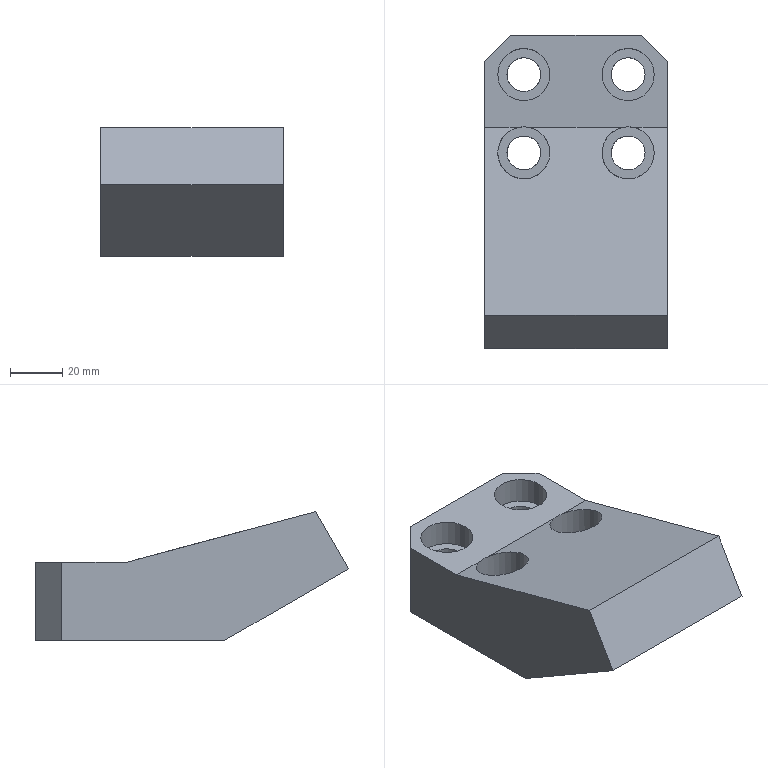Part | NX | features solid 2 | 1 solid | 22 faces | box 70 x 120.024 x 49.322 mm | volume 234951 mm3 | plane 14 | cylinder 8 | commonest cylinder face diameters 13 x4 20 x4
STEP:
#1=CARTESIAN_POINT('',(-300.,506.676,-135.678));
#2=VERTEX_POINT('',#1);
#3=CARTESIAN_POINT('',(-300.,494.007,-157.621));
#4=VERTEX_POINT('',#3);
#5=CARTESIAN_POINT('',(-300.,502.446,-143.005));
#6=DIRECTION('',(0.,0.5,0.866));
#7=VECTOR('',#6,1000.);
#8=LINE('',#5,#7);
#9=EDGE_CURVE('',#2,#4,#8,.F.);
#10=ORIENTED_EDGE('',*,*,#9,.T.);
#11=CARTESIAN_POINT('',(-300.,541.429,-185.));
#12=VERTEX_POINT('',#11);
#13=CARTESIAN_POINT('',(-300.,505.583,-164.304));
#14=DIRECTION('',(0.,-0.866,0.5));
#15=VECTOR('',#14,1000.);
#16=LINE('',#13,#15);
#17=EDGE_CURVE('',#12,#4,#16,.T.);
#18=ORIENTED_EDGE('',*,*,#17,.F.);
#19=CARTESIAN_POINT('',(-300.,604.031,-185.));
#20=VERTEX_POINT('',#19);
#21=CARTESIAN_POINT('',(-300.,581.807,-185.));
#22=DIRECTION('',(0.,1.,0.));
#23=VECTOR('',#22,1000.);
#24=LINE('',#21,#23);
#25=EDGE_CURVE('',#20,#12,#24,.F.);
#26=ORIENTED_EDGE('',*,*,#25,.F.);
#27=CARTESIAN_POINT('',(-300.,604.031,-155.));
#28=VERTEX_POINT('',#27);
#29=CARTESIAN_POINT('',(-300.,604.031,-188.825));
#30=DIRECTION('',(0.,0.,1.));
#31=VECTOR('',#30,1000.);
#32=LINE('',#29,#31);
#33=EDGE_CURVE('',#28,#20,#32,.F.);
#34=ORIENTED_EDGE('',*,*,#33,.F.);
#35=CARTESIAN_POINT('',(-300.,578.786,-155.));
#36=VERTEX_POINT('',#35);
#37=CARTESIAN_POINT('',(-300.,581.807,-155.));
#38=DIRECTION('',(0.,1.,0.));
#39=VECTOR('',#38,1000.);
#40=LINE('',#37,#39);
#41=EDGE_CURVE('',#28,#36,#40,.F.);
#42=ORIENTED_EDGE('',*,*,#41,.T.);
#43=CARTESIAN_POINT('',(-300.,590.061,-158.021));
#44=DIRECTION('',(0.,0.9659,-0.2588));
#45=VECTOR('',#44,1000.);
#46=LINE('',#43,#45);
#47=EDGE_CURVE('',#2,#36,#46,.T.);
#48=ORIENTED_EDGE('',*,*,#47,.F.);
#49=EDGE_LOOP('',(#10,#18,#26,#34,#42,#48));
#50=FACE_BOUND('',#49,.T.);
#51=CARTESIAN_POINT('',(-300.,581.807,-188.825));
#52=DIRECTION('',(1.,0.,0.));
#53=DIRECTION('',(0.,-1.,0.));
#54=AXIS2_PLACEMENT_3D('',#51,#52,#53);
#55=PLANE('',#54);
#56=ADVANCED_FACE('',(#50),#55,.T.);
#57=CARTESIAN_POINT('',(-370.,578.786,-155.));
#58=VERTEX_POINT('',#57);
#59=CARTESIAN_POINT('',(-370.,604.031,-155.));
#60=VERTEX_POINT('',#59);
#61=CARTESIAN_POINT('',(-370.,581.807,-155.));
#62=DIRECTION('',(0.,1.,0.));
#63=VECTOR('',#62,1000.);
#64=LINE('',#61,#63);
#65=EDGE_CURVE('',#58,#60,#64,.T.);
#66=ORIENTED_EDGE('',*,*,#65,.T.);
#67=CARTESIAN_POINT('',(-370.,604.031,-185.));
#68=VERTEX_POINT('',#67);
#69=CARTESIAN_POINT('',(-370.,604.031,-188.825));
#70=DIRECTION('',(0.,0.,1.));
#71=VECTOR('',#70,1000.);
#72=LINE('',#69,#71);
#73=EDGE_CURVE('',#68,#60,#72,.T.);
#74=ORIENTED_EDGE('',*,*,#73,.F.);
#75=CARTESIAN_POINT('',(-370.,541.429,-185.));
#76=VERTEX_POINT('',#75);
#77=CARTESIAN_POINT('',(-370.,581.807,-185.));
#78=DIRECTION('',(0.,1.,0.));
#79=VECTOR('',#78,1000.);
#80=LINE('',#77,#79);
#81=EDGE_CURVE('',#76,#68,#80,.T.);
#82=ORIENTED_EDGE('',*,*,#81,.F.);
#83=CARTESIAN_POINT('',(-370.,494.007,-157.621));
#84=VERTEX_POINT('',#83);
#85=CARTESIAN_POINT('',(-370.,573.369,-203.44));
#86=DIRECTION('',(0.,0.866,-0.5));
#87=VECTOR('',#86,1000.);
#88=LINE('',#85,#87);
#89=EDGE_CURVE('',#76,#84,#88,.F.);
#90=ORIENTED_EDGE('',*,*,#89,.T.);
#91=CARTESIAN_POINT('',(-370.,506.676,-135.678));
#92=VERTEX_POINT('',#91);
#93=CARTESIAN_POINT('',(-370.,502.446,-143.005));
#94=DIRECTION('',(0.,0.5,0.866));
#95=VECTOR('',#94,1000.);
#96=LINE('',#93,#95);
#97=EDGE_CURVE('',#84,#92,#96,.T.);
#98=ORIENTED_EDGE('',*,*,#97,.T.);
#99=CARTESIAN_POINT('',(-370.,590.061,-158.021));
#100=DIRECTION('',(0.,0.9659,-0.2588));
#101=VECTOR('',#100,1000.);
#102=LINE('',#99,#101);
#103=EDGE_CURVE('',#58,#92,#102,.F.);
#104=ORIENTED_EDGE('',*,*,#103,.F.);
#105=EDGE_LOOP('',(#66,#74,#82,#90,#98,#104));
#106=FACE_BOUND('',#105,.T.);
#107=CARTESIAN_POINT('',(-370.,581.807,-188.825));
#108=DIRECTION('',(1.,0.,0.));
#109=DIRECTION('',(0.,-1.,0.));
#110=AXIS2_PLACEMENT_3D('',#107,#108,#109);
#111=PLANE('',#110);
#112=ADVANCED_FACE('',(#106),#111,.F.);
#113=ORIENTED_EDGE('',*,*,#33,.T.);
#114=CARTESIAN_POINT('',(-310.,614.031,-185.));
#115=VERTEX_POINT('',#114);
#116=CARTESIAN_POINT('',(-300.,604.031,-185.));
#117=DIRECTION('',(0.7071,-0.7071,0.));
#118=VECTOR('',#117,1000.);
#119=LINE('',#116,#118);
#120=EDGE_CURVE('',#20,#115,#119,.F.);
#121=ORIENTED_EDGE('',*,*,#120,.T.);
#122=CARTESIAN_POINT('',(-310.,614.031,-155.));
#123=VERTEX_POINT('',#122);
#124=CARTESIAN_POINT('',(-310.,614.031,-188.825));
#125=DIRECTION('',(0.,0.,-1.));
#126=VECTOR('',#125,1000.);
#127=LINE('',#124,#126);
#128=EDGE_CURVE('',#115,#123,#127,.F.);
#129=ORIENTED_EDGE('',*,*,#128,.T.);
#130=CARTESIAN_POINT('',(-337.5,641.531,-155.));
#131=DIRECTION('',(-0.7071,0.7071,0.));
#132=VECTOR('',#131,1000.);
#133=LINE('',#130,#132);
#134=EDGE_CURVE('',#123,#28,#133,.F.);
#135=ORIENTED_EDGE('',*,*,#134,.T.);
#136=EDGE_LOOP('',(#113,#121,#129,#135));
#137=FACE_BOUND('',#136,.T.);
#138=CARTESIAN_POINT('',(-300.,604.031,-188.825));
#139=DIRECTION('',(-0.7071,-0.7071,0.));
#140=DIRECTION('',(-0.7071,0.7071,0.));
#141=AXIS2_PLACEMENT_3D('',#138,#139,#140);
#142=PLANE('',#141);
#143=ADVANCED_FACE('',(#137),#142,.F.);
#144=CARTESIAN_POINT('',(-360.,614.031,-155.));
#145=VERTEX_POINT('',#144);
#146=CARTESIAN_POINT('',(-360.,614.031,-155.));
#147=DIRECTION('',(-0.7071,-0.7071,0.));
#148=VECTOR('',#147,1000.);
#149=LINE('',#146,#148);
#150=EDGE_CURVE('',#145,#60,#149,.T.);
#151=ORIENTED_EDGE('',*,*,#150,.F.);
#152=CARTESIAN_POINT('',(-360.,614.031,-185.));
#153=VERTEX_POINT('',#152);
#154=CARTESIAN_POINT('',(-360.,614.031,-188.825));
#155=DIRECTION('',(0.,0.,1.));
#156=VECTOR('',#155,1000.);
#157=LINE('',#154,#156);
#158=EDGE_CURVE('',#145,#153,#157,.F.);
#159=ORIENTED_EDGE('',*,*,#158,.T.);
#160=CARTESIAN_POINT('',(-360.,614.031,-185.));
#161=DIRECTION('',(-0.7071,-0.7071,0.));
#162=VECTOR('',#161,1000.);
#163=LINE('',#160,#162);
#164=EDGE_CURVE('',#153,#68,#163,.T.);
#165=ORIENTED_EDGE('',*,*,#164,.T.);
#166=ORIENTED_EDGE('',*,*,#73,.T.);
#167=EDGE_LOOP('',(#151,#159,#165,#166));
#168=FACE_BOUND('',#167,.T.);
#169=CARTESIAN_POINT('',(-360.,614.031,-188.825));
#170=DIRECTION('',(-0.7071,0.7071,0.));
#171=DIRECTION('',(0.7071,0.7071,0.));
#172=AXIS2_PLACEMENT_3D('',#169,#170,#171);
#173=PLANE('',#172);
#174=ADVANCED_FACE('',(#168),#173,.T.);
#175=CARTESIAN_POINT('',(-345.,599.031,-165.));
#176=VERTEX_POINT('',#175);
#177=CARTESIAN_POINT('',(-355.,599.031,-165.));
#178=DIRECTION('',(0.,0.,1.));
#179=DIRECTION('',(1.,0.,0.));
#180=AXIS2_PLACEMENT_3D('',#177,#178,#179);
#181=CIRCLE('',#180,10.);
#182=EDGE_CURVE('',#176,#176,#181,.F.);
#183=ORIENTED_EDGE('',*,*,#182,.T.);
#184=EDGE_LOOP('',(#183));
#185=FACE_BOUND('',#184,.T.);
#186=CARTESIAN_POINT('',(-365.,599.031,-155.));
#187=VERTEX_POINT('',#186);
#188=CARTESIAN_POINT('',(-355.,599.031,-155.));
#189=DIRECTION('',(0.,0.,-1.));
#190=DIRECTION('',(-1.,0.,0.));
#191=AXIS2_PLACEMENT_3D('',#188,#189,#190);
#192=CIRCLE('',#191,10.);
#193=EDGE_CURVE('',#187,#187,#192,.T.);
#194=ORIENTED_EDGE('',*,*,#193,.F.);
#195=EDGE_LOOP('',(#194));
#196=FACE_BOUND('',#195,.T.);
#197=CARTESIAN_POINT('',(-355.,599.031,15.));
#198=DIRECTION('',(0.,0.,-1.));
#199=DIRECTION('',(0.,1.,0.));
#200=AXIS2_PLACEMENT_3D('',#197,#198,#199);
#201=CYLINDRICAL_SURFACE('',#200,10.);
#202=ADVANCED_FACE('',(#185,#196),#201,.F.);
#203=CARTESIAN_POINT('',(-305.,599.031,-165.));
#204=VERTEX_POINT('',#203);
#205=CARTESIAN_POINT('',(-315.,599.031,-165.));
#206=DIRECTION('',(0.,0.,1.));
#207=DIRECTION('',(1.,0.,0.));
#208=AXIS2_PLACEMENT_3D('',#205,#206,#207);
#209=CIRCLE('',#208,10.);
#210=EDGE_CURVE('',#204,#204,#209,.F.);
#211=ORIENTED_EDGE('',*,*,#210,.T.);
#212=EDGE_LOOP('',(#211));
#213=FACE_BOUND('',#212,.T.);
#214=CARTESIAN_POINT('',(-325.,599.031,-155.));
#215=VERTEX_POINT('',#214);
#216=CARTESIAN_POINT('',(-315.,599.031,-155.));
#217=DIRECTION('',(0.,0.,-1.));
#218=DIRECTION('',(-1.,0.,0.));
#219=AXIS2_PLACEMENT_3D('',#216,#217,#218);
#220=CIRCLE('',#219,10.);
#221=EDGE_CURVE('',#215,#215,#220,.T.);
#222=ORIENTED_EDGE('',*,*,#221,.F.);
#223=EDGE_LOOP('',(#222));
#224=FACE_BOUND('',#223,.T.);
#225=CARTESIAN_POINT('',(-315.,599.031,15.));
#226=DIRECTION('',(0.,0.,-1.));
#227=DIRECTION('',(0.,1.,0.));
#228=AXIS2_PLACEMENT_3D('',#225,#226,#227);
#229=CYLINDRICAL_SURFACE('',#228,10.);
#230=ADVANCED_FACE('',(#213,#224),#229,.F.);
#231=CARTESIAN_POINT('',(-305.,569.031,-165.));
#232=VERTEX_POINT('',#231);
#233=CARTESIAN_POINT('',(-315.,569.031,-165.));
#234=DIRECTION('',(0.,0.,1.));
#235=DIRECTION('',(1.,0.,0.));
#236=AXIS2_PLACEMENT_3D('',#233,#234,#235);
#237=CIRCLE('',#236,10.);
#238=EDGE_CURVE('',#232,#232,#237,.F.);
#239=ORIENTED_EDGE('',*,*,#238,.T.);
#240=EDGE_LOOP('',(#239));
#241=FACE_BOUND('',#240,.T.);
#242=CARTESIAN_POINT('',(-312.801,578.786,-155.));
#243=VERTEX_POINT('',#242);
#244=CARTESIAN_POINT('',(-317.199,578.786,-155.));
#245=VERTEX_POINT('',#244);
#246=CARTESIAN_POINT('',(-315.,569.031,-152.386));
#247=DIRECTION('',(0.,-0.2588,-0.9659));
#248=DIRECTION('',(0.,0.9659,-0.2588));
#249=AXIS2_PLACEMENT_3D('',#246,#247,#248);
#250=ELLIPSE('',#249,10.353,10.);
#251=EDGE_CURVE('',#243,#245,#250,.T.);
#252=ORIENTED_EDGE('',*,*,#251,.F.);
#253=CARTESIAN_POINT('',(-315.,569.031,-155.));
#254=DIRECTION('',(0.,0.,-1.));
#255=DIRECTION('',(-1.,0.,0.));
#256=AXIS2_PLACEMENT_3D('',#253,#254,#255);
#257=CIRCLE('',#256,10.);
#258=EDGE_CURVE('',#243,#245,#257,.F.);
#259=ORIENTED_EDGE('',*,*,#258,.T.);
#260=EDGE_LOOP('',(#252,#259));
#261=FACE_BOUND('',#260,.T.);
#262=CARTESIAN_POINT('',(-315.,569.031,15.));
#263=DIRECTION('',(0.,0.,-1.));
#264=DIRECTION('',(0.,1.,0.));
#265=AXIS2_PLACEMENT_3D('',#262,#263,#264);
#266=CYLINDRICAL_SURFACE('',#265,10.);
#267=ADVANCED_FACE('',(#241,#261),#266,.F.);
#268=CARTESIAN_POINT('',(-345.,569.031,-165.));
#269=VERTEX_POINT('',#268);
#270=CARTESIAN_POINT('',(-355.,569.031,-165.));
#271=DIRECTION('',(0.,0.,1.));
#272=DIRECTION('',(1.,0.,0.));
#273=AXIS2_PLACEMENT_3D('',#270,#271,#272);
#274=CIRCLE('',#273,10.);
#275=EDGE_CURVE('',#269,#269,#274,.F.);
#276=ORIENTED_EDGE('',*,*,#275,.T.);
#277=EDGE_LOOP('',(#276));
#278=FACE_BOUND('',#277,.T.);
#279=CARTESIAN_POINT('',(-352.801,578.786,-155.));
#280=VERTEX_POINT('',#279);
#281=CARTESIAN_POINT('',(-357.199,578.786,-155.));
#282=VERTEX_POINT('',#281);
#283=CARTESIAN_POINT('',(-355.,569.031,-152.386));
#284=DIRECTION('',(0.,-0.2588,-0.9659));
#285=DIRECTION('',(0.,0.9659,-0.2588));
#286=AXIS2_PLACEMENT_3D('',#283,#284,#285);
#287=ELLIPSE('',#286,10.353,10.);
#288=EDGE_CURVE('',#280,#282,#287,.T.);
#289=ORIENTED_EDGE('',*,*,#288,.F.);
#290=CARTESIAN_POINT('',(-355.,569.031,-155.));
#291=DIRECTION('',(0.,0.,-1.));
#292=DIRECTION('',(-1.,0.,0.));
#293=AXIS2_PLACEMENT_3D('',#290,#291,#292);
#294=CIRCLE('',#293,10.);
#295=EDGE_CURVE('',#280,#282,#294,.F.);
#296=ORIENTED_EDGE('',*,*,#295,.T.);
#297=EDGE_LOOP('',(#289,#296));
#298=FACE_BOUND('',#297,.T.);
#299=CARTESIAN_POINT('',(-355.,569.031,15.));
#300=DIRECTION('',(0.,0.,-1.));
#301=DIRECTION('',(0.,1.,0.));
#302=AXIS2_PLACEMENT_3D('',#299,#300,#301);
#303=CYLINDRICAL_SURFACE('',#302,10.);
#304=ADVANCED_FACE('',(#278,#298),#303,.F.);
#305=CARTESIAN_POINT('',(-355.,562.531,-185.));
#306=VERTEX_POINT('',#305);
#307=CARTESIAN_POINT('',(-355.,569.031,-185.));
#308=DIRECTION('',(0.,0.,-1.));
#309=DIRECTION('',(0.,-1.,0.));
#310=AXIS2_PLACEMENT_3D('',#307,#308,#309);
#311=CIRCLE('',#310,6.5);
#312=EDGE_CURVE('',#306,#306,#311,.T.);
#313=ORIENTED_EDGE('',*,*,#312,.T.);
#314=EDGE_LOOP('',(#313));
#315=FACE_BOUND('',#314,.T.);
#316=CARTESIAN_POINT('',(-348.5,569.031,-165.));
#317=VERTEX_POINT('',#316);
#318=CARTESIAN_POINT('',(-355.,569.031,-165.));
#319=DIRECTION('',(0.,0.,1.));
#320=DIRECTION('',(1.,0.,0.));
#321=AXIS2_PLACEMENT_3D('',#318,#319,#320);
#322=CIRCLE('',#321,6.5);
#323=EDGE_CURVE('',#317,#317,#322,.T.);
#324=ORIENTED_EDGE('',*,*,#323,.T.);
#325=EDGE_LOOP('',(#324));
#326=FACE_BOUND('',#325,.T.);
#327=CARTESIAN_POINT('',(-355.,569.031,-135.));
#328=DIRECTION('',(0.,0.,-1.));
#329=DIRECTION('',(0.,1.,0.));
#330=AXIS2_PLACEMENT_3D('',#327,#328,#329);
#331=CYLINDRICAL_SURFACE('',#330,6.5);
#332=ADVANCED_FACE('',(#315,#326),#331,.F.);
#333=CARTESIAN_POINT('',(-315.,562.531,-185.));
#334=VERTEX_POINT('',#333);
#335=CARTESIAN_POINT('',(-315.,569.031,-185.));
#336=DIRECTION('',(0.,0.,-1.));
#337=DIRECTION('',(0.,-1.,0.));
#338=AXIS2_PLACEMENT_3D('',#335,#336,#337);
#339=CIRCLE('',#338,6.5);
#340=EDGE_CURVE('',#334,#334,#339,.T.);
#341=ORIENTED_EDGE('',*,*,#340,.T.);
#342=EDGE_LOOP('',(#341));
#343=FACE_BOUND('',#342,.T.);
#344=CARTESIAN_POINT('',(-308.5,569.031,-165.));
#345=VERTEX_POINT('',#344);
#346=CARTESIAN_POINT('',(-315.,569.031,-165.));
#347=DIRECTION('',(0.,0.,1.));
#348=DIRECTION('',(1.,0.,0.));
#349=AXIS2_PLACEMENT_3D('',#346,#347,#348);
#350=CIRCLE('',#349,6.5);
#351=EDGE_CURVE('',#345,#345,#350,.T.);
#352=ORIENTED_EDGE('',*,*,#351,.T.);
#353=EDGE_LOOP('',(#352));
#354=FACE_BOUND('',#353,.T.);
#355=CARTESIAN_POINT('',(-315.,569.031,-135.));
#356=DIRECTION('',(0.,0.,-1.));
#357=DIRECTION('',(0.,1.,0.));
#358=AXIS2_PLACEMENT_3D('',#355,#356,#357);
#359=CYLINDRICAL_SURFACE('',#358,6.5);
#360=ADVANCED_FACE('',(#343,#354),#359,.F.);
#361=CARTESIAN_POINT('',(-315.,592.531,-185.));
#362=VERTEX_POINT('',#361);
#363=CARTESIAN_POINT('',(-315.,599.031,-185.));
#364=DIRECTION('',(0.,0.,-1.));
#365=DIRECTION('',(0.,-1.,0.));
#366=AXIS2_PLACEMENT_3D('',#363,#364,#365);
#367=CIRCLE('',#366,6.5);
#368=EDGE_CURVE('',#362,#362,#367,.T.);
#369=ORIENTED_EDGE('',*,*,#368,.T.);
#370=EDGE_LOOP('',(#369));
#371=FACE_BOUND('',#370,.T.);
#372=CARTESIAN_POINT('',(-308.5,599.031,-165.));
#373=VERTEX_POINT('',#372);
#374=CARTESIAN_POINT('',(-315.,599.031,-165.));
#375=DIRECTION('',(0.,0.,1.));
#376=DIRECTION('',(1.,0.,0.));
#377=AXIS2_PLACEMENT_3D('',#374,#375,#376);
#378=CIRCLE('',#377,6.5);
#379=EDGE_CURVE('',#373,#373,#378,.T.);
#380=ORIENTED_EDGE('',*,*,#379,.T.);
#381=EDGE_LOOP('',(#380));
#382=FACE_BOUND('',#381,.T.);
#383=CARTESIAN_POINT('',(-315.,599.031,-135.));
#384=DIRECTION('',(0.,0.,-1.));
#385=DIRECTION('',(0.,1.,0.));
#386=AXIS2_PLACEMENT_3D('',#383,#384,#385);
#387=CYLINDRICAL_SURFACE('',#386,6.5);
#388=ADVANCED_FACE('',(#371,#382),#387,.F.);
#389=CARTESIAN_POINT('',(-355.,592.531,-185.));
#390=VERTEX_POINT('',#389);
#391=CARTESIAN_POINT('',(-355.,599.031,-185.));
#392=DIRECTION('',(0.,0.,-1.));
#393=DIRECTION('',(0.,-1.,0.));
#394=AXIS2_PLACEMENT_3D('',#391,#392,#393);
#395=CIRCLE('',#394,6.5);
#396=EDGE_CURVE('',#390,#390,#395,.T.);
#397=ORIENTED_EDGE('',*,*,#396,.T.);
#398=EDGE_LOOP('',(#397));
#399=FACE_BOUND('',#398,.T.);
#400=CARTESIAN_POINT('',(-348.5,599.031,-165.));
#401=VERTEX_POINT('',#400);
#402=CARTESIAN_POINT('',(-355.,599.031,-165.));
#403=DIRECTION('',(0.,0.,1.));
#404=DIRECTION('',(1.,0.,0.));
#405=AXIS2_PLACEMENT_3D('',#402,#403,#404);
#406=CIRCLE('',#405,6.5);
#407=EDGE_CURVE('',#401,#401,#406,.T.);
#408=ORIENTED_EDGE('',*,*,#407,.T.);
#409=EDGE_LOOP('',(#408));
#410=FACE_BOUND('',#409,.T.);
#411=CARTESIAN_POINT('',(-355.,599.031,-135.));
#412=DIRECTION('',(0.,0.,-1.));
#413=DIRECTION('',(0.,1.,0.));
#414=AXIS2_PLACEMENT_3D('',#411,#412,#413);
#415=CYLINDRICAL_SURFACE('',#414,6.5);
#416=ADVANCED_FACE('',(#399,#410),#415,.F.);
#417=CARTESIAN_POINT('',(-355.,614.031,-185.));
#418=DIRECTION('',(-1.,0.,0.));
#419=VECTOR('',#418,1000.);
#420=LINE('',#417,#419);
#421=EDGE_CURVE('',#153,#115,#420,.F.);
#422=ORIENTED_EDGE('',*,*,#421,.F.);
#423=ORIENTED_EDGE('',*,*,#158,.F.);
#424=CARTESIAN_POINT('',(-355.,614.031,-155.));
#425=DIRECTION('',(1.,0.,0.));
#426=VECTOR('',#425,1000.);
#427=LINE('',#424,#426);
#428=EDGE_CURVE('',#123,#145,#427,.F.);
#429=ORIENTED_EDGE('',*,*,#428,.F.);
#430=ORIENTED_EDGE('',*,*,#128,.F.);
#431=EDGE_LOOP('',(#422,#423,#429,#430));
#432=FACE_BOUND('',#431,.T.);
#433=CARTESIAN_POINT('',(-355.,614.031,-188.825));
#434=DIRECTION('',(0.,1.,0.));
#435=DIRECTION('',(1.,0.,0.));
#436=AXIS2_PLACEMENT_3D('',#433,#434,#435);
#437=PLANE('',#436);
#438=ADVANCED_FACE('',(#432),#437,.T.);
#439=ORIENTED_EDGE('',*,*,#368,.F.);
#440=EDGE_LOOP('',(#439));
#441=FACE_BOUND('',#440,.T.);
#442=ORIENTED_EDGE('',*,*,#396,.F.);
#443=EDGE_LOOP('',(#442));
#444=FACE_BOUND('',#443,.T.);
#445=ORIENTED_EDGE('',*,*,#25,.T.);
#446=CARTESIAN_POINT('',(-23.,541.429,-185.));
#447=DIRECTION('',(1.,0.,0.));
#448=VECTOR('',#447,1000.);
#449=LINE('',#446,#448);
#450=EDGE_CURVE('',#12,#76,#449,.F.);
#451=ORIENTED_EDGE('',*,*,#450,.T.);
#452=ORIENTED_EDGE('',*,*,#81,.T.);
#453=ORIENTED_EDGE('',*,*,#164,.F.);
#454=ORIENTED_EDGE('',*,*,#421,.T.);
#455=ORIENTED_EDGE('',*,*,#120,.F.);
#456=EDGE_LOOP('',(#445,#451,#452,#453,#454,#455));
#457=FACE_BOUND('',#456,.T.);
#458=ORIENTED_EDGE('',*,*,#340,.F.);
#459=EDGE_LOOP('',(#458));
#460=FACE_BOUND('',#459,.T.);
#461=ORIENTED_EDGE('',*,*,#312,.F.);
#462=EDGE_LOOP('',(#461));
#463=FACE_BOUND('',#462,.T.);
#464=CARTESIAN_POINT('',(-23.,171.031,-185.));
#465=DIRECTION('',(0.,0.,1.));
#466=DIRECTION('',(0.,-1.,0.));
#467=AXIS2_PLACEMENT_3D('',#464,#465,#466);
#468=PLANE('',#467);
#469=ADVANCED_FACE('',(#441,#444,#457,#460,#463),#468,.F.);
#470=ORIENTED_EDGE('',*,*,#182,.F.);
#471=EDGE_LOOP('',(#470));
#472=FACE_BOUND('',#471,.T.);
#473=ORIENTED_EDGE('',*,*,#407,.F.);
#474=EDGE_LOOP('',(#473));
#475=FACE_BOUND('',#474,.T.);
#476=CARTESIAN_POINT('',(-355.,599.031,-165.));
#477=DIRECTION('',(0.,0.,1.));
#478=DIRECTION('',(0.,-1.,0.));
#479=AXIS2_PLACEMENT_3D('',#476,#477,#478);
#480=PLANE('',#479);
#481=ADVANCED_FACE('',(#472,#475),#480,.T.);
#482=ORIENTED_EDGE('',*,*,#210,.F.);
#483=EDGE_LOOP('',(#482));
#484=FACE_BOUND('',#483,.T.);
#485=ORIENTED_EDGE('',*,*,#379,.F.);
#486=EDGE_LOOP('',(#485));
#487=FACE_BOUND('',#486,.T.);
#488=CARTESIAN_POINT('',(-315.,599.031,-165.));
#489=DIRECTION('',(0.,0.,1.));
#490=DIRECTION('',(0.,-1.,0.));
#491=AXIS2_PLACEMENT_3D('',#488,#489,#490);
#492=PLANE('',#491);
#493=ADVANCED_FACE('',(#484,#487),#492,.T.);
#494=ORIENTED_EDGE('',*,*,#238,.F.);
#495=EDGE_LOOP('',(#494));
#496=FACE_BOUND('',#495,.T.);
#497=ORIENTED_EDGE('',*,*,#351,.F.);
#498=EDGE_LOOP('',(#497));
#499=FACE_BOUND('',#498,.T.);
#500=CARTESIAN_POINT('',(-315.,569.031,-165.));
#501=DIRECTION('',(0.,0.,1.));
#502=DIRECTION('',(0.,-1.,0.));
#503=AXIS2_PLACEMENT_3D('',#500,#501,#502);
#504=PLANE('',#503);
#505=ADVANCED_FACE('',(#496,#499),#504,.T.);
#506=ORIENTED_EDGE('',*,*,#275,.F.);
#507=EDGE_LOOP('',(#506));
#508=FACE_BOUND('',#507,.T.);
#509=ORIENTED_EDGE('',*,*,#323,.F.);
#510=EDGE_LOOP('',(#509));
#511=FACE_BOUND('',#510,.T.);
#512=CARTESIAN_POINT('',(-355.,569.031,-165.));
#513=DIRECTION('',(0.,0.,1.));
#514=DIRECTION('',(0.,-1.,0.));
#515=AXIS2_PLACEMENT_3D('',#512,#513,#514);
#516=PLANE('',#515);
#517=ADVANCED_FACE('',(#508,#511),#516,.T.);
#518=ORIENTED_EDGE('',*,*,#450,.F.);
#519=ORIENTED_EDGE('',*,*,#17,.T.);
#520=CARTESIAN_POINT('',(-335.,494.007,-157.621));
#521=DIRECTION('',(1.,0.,0.));
#522=VECTOR('',#521,1000.);
#523=LINE('',#520,#522);
#524=EDGE_CURVE('',#4,#84,#523,.F.);
#525=ORIENTED_EDGE('',*,*,#524,.T.);
#526=ORIENTED_EDGE('',*,*,#89,.F.);
#527=EDGE_LOOP('',(#518,#519,#525,#526));
#528=FACE_BOUND('',#527,.T.);
#529=CARTESIAN_POINT('',(-335.,505.583,-164.304));
#530=DIRECTION('',(0.,0.5,0.866));
#531=DIRECTION('',(0.,0.866,-0.5));
#532=AXIS2_PLACEMENT_3D('',#529,#530,#531);
#533=PLANE('',#532);
#534=ADVANCED_FACE('',(#528),#533,.F.);
#535=ORIENTED_EDGE('',*,*,#97,.F.);
#536=ORIENTED_EDGE('',*,*,#524,.F.);
#537=ORIENTED_EDGE('',*,*,#9,.F.);
#538=CARTESIAN_POINT('',(-335.,506.676,-135.678));
#539=DIRECTION('',(-1.,0.,0.));
#540=VECTOR('',#539,1000.);
#541=LINE('',#538,#540);
#542=EDGE_CURVE('',#92,#2,#541,.F.);
#543=ORIENTED_EDGE('',*,*,#542,.F.);
#544=EDGE_LOOP('',(#535,#536,#537,#543));
#545=FACE_BOUND('',#544,.T.);
#546=CARTESIAN_POINT('',(-335.,502.838,-142.326));
#547=DIRECTION('',(0.,-0.866,0.5));
#548=DIRECTION('',(-1.,0.,0.));
#549=AXIS2_PLACEMENT_3D('',#546,#547,#548);
#550=PLANE('',#549);
#551=ADVANCED_FACE('',(#545),#550,.T.);
#552=ORIENTED_EDGE('',*,*,#41,.F.);
#553=ORIENTED_EDGE('',*,*,#134,.F.);
#554=ORIENTED_EDGE('',*,*,#428,.T.);
#555=ORIENTED_EDGE('',*,*,#150,.T.);
#556=ORIENTED_EDGE('',*,*,#65,.F.);
#557=CARTESIAN_POINT('',(-355.,578.786,-155.));
#558=DIRECTION('',(1.,0.,0.));
#559=VECTOR('',#558,1000.);
#560=LINE('',#557,#559);
#561=EDGE_CURVE('',#282,#58,#560,.F.);
#562=ORIENTED_EDGE('',*,*,#561,.F.);
#563=ORIENTED_EDGE('',*,*,#295,.F.);
#564=CARTESIAN_POINT('',(-355.,578.786,-155.));
#565=DIRECTION('',(1.,0.,0.));
#566=VECTOR('',#565,1000.);
#567=LINE('',#564,#566);
#568=EDGE_CURVE('',#245,#280,#567,.F.);
#569=ORIENTED_EDGE('',*,*,#568,.F.);
#570=ORIENTED_EDGE('',*,*,#258,.F.);
#571=CARTESIAN_POINT('',(-355.,578.786,-155.));
#572=DIRECTION('',(1.,0.,0.));
#573=VECTOR('',#572,1000.);
#574=LINE('',#571,#573);
#575=EDGE_CURVE('',#36,#243,#574,.F.);
#576=ORIENTED_EDGE('',*,*,#575,.F.);
#577=EDGE_LOOP('',(#552,#553,#554,#555,#556,#562,#563,#569,#570,#576));
#578=FACE_BOUND('',#577,.T.);
#579=ORIENTED_EDGE('',*,*,#193,.T.);
#580=EDGE_LOOP('',(#579));
#581=FACE_BOUND('',#580,.T.);
#582=ORIENTED_EDGE('',*,*,#221,.T.);
#583=EDGE_LOOP('',(#582));
#584=FACE_BOUND('',#583,.T.);
#585=CARTESIAN_POINT('',(-355.,624.031,-155.));
#586=DIRECTION('',(0.,0.,1.));
#587=DIRECTION('',(-1.,0.,0.));
#588=AXIS2_PLACEMENT_3D('',#585,#586,#587);
#589=PLANE('',#588);
#590=ADVANCED_FACE('',(#578,#581,#584),#589,.T.);
#591=ORIENTED_EDGE('',*,*,#103,.T.);
#592=ORIENTED_EDGE('',*,*,#542,.T.);
#593=ORIENTED_EDGE('',*,*,#47,.T.);
#594=ORIENTED_EDGE('',*,*,#575,.T.);
#595=ORIENTED_EDGE('',*,*,#251,.T.);
#596=ORIENTED_EDGE('',*,*,#568,.T.);
#597=ORIENTED_EDGE('',*,*,#288,.T.);
#598=ORIENTED_EDGE('',*,*,#561,.T.);
#599=EDGE_LOOP('',(#591,#592,#593,#594,#595,#596,#597,#598));
#600=FACE_BOUND('',#599,.T.);
#601=CARTESIAN_POINT('',(-335.,542.102,-145.17));
#602=DIRECTION('',(0.,0.2588,0.9659));
#603=DIRECTION('',(0.,-0.9659,0.2588));
#604=AXIS2_PLACEMENT_3D('',#601,#602,#603);
#605=PLANE('',#604);
#606=ADVANCED_FACE('',(#600),#605,.T.);
#607=CLOSED_SHELL('',(#56,#112,#143,#174,#202,#230,#267,#304,#332,#360,#388,#416,#438,#469,#481,#493,#505,#517,#534,#551,#590,#606));
#608=MANIFOLD_SOLID_BREP('',#607);
#609=(LENGTH_UNIT()NAMED_UNIT(*)SI_UNIT(.MILLI.,.METRE.));
#610=UNCERTAINTY_MEASURE_WITH_UNIT(LENGTH_MEASURE(0.00001),#609,'','');
#611=(NAMED_UNIT(*)PLANE_ANGLE_UNIT()SI_UNIT($,.RADIAN.));
#612=(NAMED_UNIT(*)SI_UNIT($,.STERADIAN.)SOLID_ANGLE_UNIT());
#613=(GEOMETRIC_REPRESENTATION_CONTEXT(3)GLOBAL_UNCERTAINTY_ASSIGNED_CONTEXT((#610))GLOBAL_UNIT_ASSIGNED_CONTEXT((#609,#611,#612))REPRESENTATION_CONTEXT('',''));
#614=ADVANCED_BREP_SHAPE_REPRESENTATION('',(#608),#613);